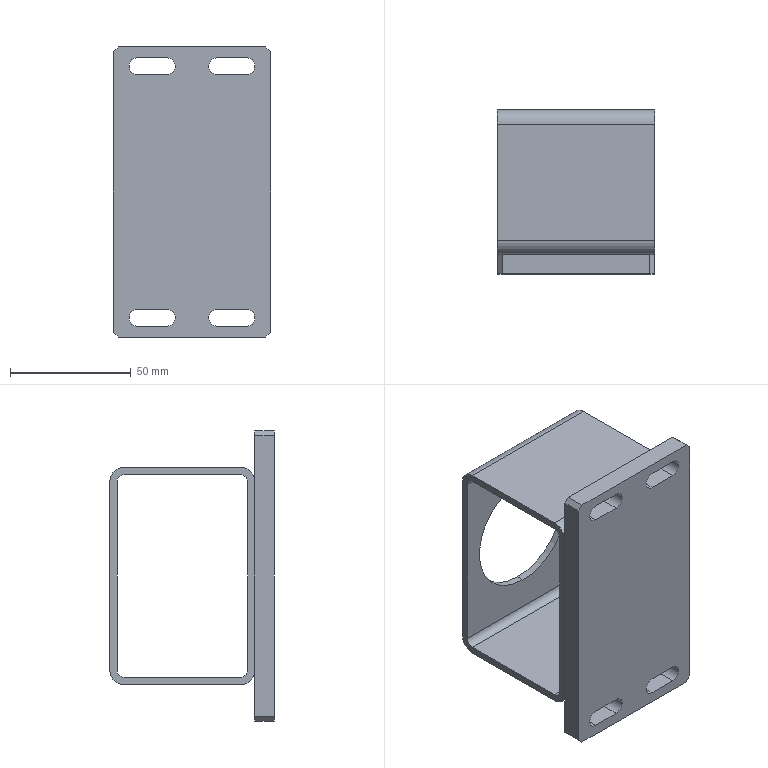Part | SolidWorks | features ICE 5, MirrorPattern 3, Chamfer 1, WeldMemberFeat 1, WeldmentFeature 1 | 2 solids | 46 faces | box 65 x 68 x 120 mm | volume 106942 mm3 | plane 28 | cylinder 18 | commonest cylinder face diameters 7 x8 6 x4 12 x4 51 x2
STEP:
#1=CARTESIAN_POINT('',(0.,27.,-25.5));
#2=VERTEX_POINT('',#1);
#3=CARTESIAN_POINT('',(0.,27.,25.5));
#4=VERTEX_POINT('',#3);
#5=CARTESIAN_POINT('',(0.,27.,0.));
#6=DIRECTION('',(0.,1.,0.));
#7=DIRECTION('',(1.,0.,0.));
#8=AXIS2_PLACEMENT_3D('',#5,#6,#7);
#9=CIRCLE('',#8,25.5);
#10=EDGE_CURVE('',#2,#4,#9,.T.);
#11=ORIENTED_EDGE('',*,*,#10,.F.);
#12=CARTESIAN_POINT('',(0.,30.,-25.5));
#13=VERTEX_POINT('',#12);
#14=CARTESIAN_POINT('',(0.,-30.001,-25.5));
#15=DIRECTION('',(0.,1.,0.));
#16=VECTOR('',#15,1000.);
#17=LINE('',#14,#16);
#18=EDGE_CURVE('',#2,#13,#17,.T.);
#19=ORIENTED_EDGE('',*,*,#18,.T.);
#20=CARTESIAN_POINT('',(0.,30.,25.5));
#21=VERTEX_POINT('',#20);
#22=CARTESIAN_POINT('',(0.,30.,0.));
#23=DIRECTION('',(0.,1.,0.));
#24=DIRECTION('',(0.,0.,1.));
#25=AXIS2_PLACEMENT_3D('',#22,#23,#24);
#26=CIRCLE('',#25,25.5);
#27=EDGE_CURVE('',#13,#21,#26,.T.);
#28=ORIENTED_EDGE('',*,*,#27,.T.);
#29=CARTESIAN_POINT('',(0.,-30.001,25.5));
#30=DIRECTION('',(0.,1.,0.));
#31=VECTOR('',#30,1000.);
#32=LINE('',#29,#31);
#33=EDGE_CURVE('',#4,#21,#32,.T.);
#34=ORIENTED_EDGE('',*,*,#33,.F.);
#35=EDGE_LOOP('',(#11,#19,#28,#34));
#36=FACE_OUTER_BOUND('',#35,.T.);
#37=CARTESIAN_POINT('',(0.,-30.001,0.));
#38=DIRECTION('',(0.,1.,0.));
#39=DIRECTION('',(0.,0.,1.));
#40=AXIS2_PLACEMENT_3D('',#37,#38,#39);
#41=CYLINDRICAL_SURFACE('',#40,25.5);
#42=ADVANCED_FACE('',(#36),#41,.F.);
#43=CARTESIAN_POINT('',(-32.5,30.,39.));
#44=VERTEX_POINT('',#43);
#45=CARTESIAN_POINT('',(-32.5,24.,45.));
#46=VERTEX_POINT('',#45);
#47=CARTESIAN_POINT('',(-32.5,24.,39.));
#48=DIRECTION('',(1.,0.,0.));
#49=DIRECTION('',(0.,1.,0.));
#50=AXIS2_PLACEMENT_3D('',#47,#48,#49);
#51=CIRCLE('',#50,6.);
#52=EDGE_CURVE('',#44,#46,#51,.T.);
#53=ORIENTED_EDGE('',*,*,#52,.T.);
#54=CARTESIAN_POINT('',(32.5,24.,45.));
#55=VERTEX_POINT('',#54);
#56=CARTESIAN_POINT('',(32.5,24.,45.));
#57=DIRECTION('',(-1.,0.,0.));
#58=VECTOR('',#57,1000.);
#59=LINE('',#56,#58);
#60=EDGE_CURVE('',#55,#46,#59,.T.);
#61=ORIENTED_EDGE('',*,*,#60,.F.);
#62=CARTESIAN_POINT('',(32.5,30.,39.));
#63=VERTEX_POINT('',#62);
#64=CARTESIAN_POINT('',(32.5,24.,39.));
#65=DIRECTION('',(1.,0.,0.));
#66=DIRECTION('',(0.,1.,0.));
#67=AXIS2_PLACEMENT_3D('',#64,#65,#66);
#68=CIRCLE('',#67,6.);
#69=EDGE_CURVE('',#63,#55,#68,.T.);
#70=ORIENTED_EDGE('',*,*,#69,.F.);
#71=CARTESIAN_POINT('',(32.5,30.,39.));
#72=DIRECTION('',(-1.,0.,0.));
#73=VECTOR('',#72,1000.);
#74=LINE('',#71,#73);
#75=EDGE_CURVE('',#63,#44,#74,.T.);
#76=ORIENTED_EDGE('',*,*,#75,.T.);
#77=EDGE_LOOP('',(#53,#61,#70,#76));
#78=FACE_OUTER_BOUND('',#77,.T.);
#79=CARTESIAN_POINT('',(32.5,24.,39.));
#80=DIRECTION('',(-1.,0.,0.));
#81=DIRECTION('',(0.,-1.,0.));
#82=AXIS2_PLACEMENT_3D('',#79,#80,#81);
#83=CYLINDRICAL_SURFACE('',#82,6.);
#84=ADVANCED_FACE('',(#78),#83,.T.);
#85=CARTESIAN_POINT('',(-32.5,-24.,45.));
#86=VERTEX_POINT('',#85);
#87=CARTESIAN_POINT('',(-32.5,24.,45.));
#88=DIRECTION('',(0.,-1.,0.));
#89=VECTOR('',#88,1000.);
#90=LINE('',#87,#89);
#91=EDGE_CURVE('',#46,#86,#90,.T.);
#92=ORIENTED_EDGE('',*,*,#91,.T.);
#93=CARTESIAN_POINT('',(32.5,-24.,45.));
#94=VERTEX_POINT('',#93);
#95=CARTESIAN_POINT('',(32.5,-24.,45.));
#96=DIRECTION('',(-1.,0.,0.));
#97=VECTOR('',#96,1000.);
#98=LINE('',#95,#97);
#99=EDGE_CURVE('',#94,#86,#98,.T.);
#100=ORIENTED_EDGE('',*,*,#99,.F.);
#101=CARTESIAN_POINT('',(32.5,24.,45.));
#102=DIRECTION('',(0.,-1.,0.));
#103=VECTOR('',#102,1000.);
#104=LINE('',#101,#103);
#105=EDGE_CURVE('',#55,#94,#104,.T.);
#106=ORIENTED_EDGE('',*,*,#105,.F.);
#107=ORIENTED_EDGE('',*,*,#60,.T.);
#108=EDGE_LOOP('',(#92,#100,#106,#107));
#109=FACE_OUTER_BOUND('',#108,.T.);
#110=CARTESIAN_POINT('',(32.5,24.,45.));
#111=DIRECTION('',(0.,0.,-1.));
#112=DIRECTION('',(-1.,0.,0.));
#113=AXIS2_PLACEMENT_3D('',#110,#111,#112);
#114=PLANE('',#113);
#115=ADVANCED_FACE('',(#109),#114,.F.);
#116=CARTESIAN_POINT('',(-32.5,-30.,39.));
#117=VERTEX_POINT('',#116);
#118=CARTESIAN_POINT('',(-32.5,-24.,39.));
#119=DIRECTION('',(1.,0.,0.));
#120=DIRECTION('',(0.,1.,0.));
#121=AXIS2_PLACEMENT_3D('',#118,#119,#120);
#122=CIRCLE('',#121,6.);
#123=EDGE_CURVE('',#86,#117,#122,.T.);
#124=ORIENTED_EDGE('',*,*,#123,.T.);
#125=CARTESIAN_POINT('',(32.5,-30.,39.));
#126=VERTEX_POINT('',#125);
#127=CARTESIAN_POINT('',(32.5,-30.,39.));
#128=DIRECTION('',(-1.,0.,0.));
#129=VECTOR('',#128,1000.);
#130=LINE('',#127,#129);
#131=EDGE_CURVE('',#126,#117,#130,.T.);
#132=ORIENTED_EDGE('',*,*,#131,.F.);
#133=CARTESIAN_POINT('',(32.5,-24.,39.));
#134=DIRECTION('',(1.,0.,0.));
#135=DIRECTION('',(0.,1.,0.));
#136=AXIS2_PLACEMENT_3D('',#133,#134,#135);
#137=CIRCLE('',#136,6.);
#138=EDGE_CURVE('',#94,#126,#137,.T.);
#139=ORIENTED_EDGE('',*,*,#138,.F.);
#140=ORIENTED_EDGE('',*,*,#99,.T.);
#141=EDGE_LOOP('',(#124,#132,#139,#140));
#142=FACE_OUTER_BOUND('',#141,.T.);
#143=CARTESIAN_POINT('',(32.5,-24.,39.));
#144=DIRECTION('',(-1.,0.,0.));
#145=DIRECTION('',(0.,-1.,0.));
#146=AXIS2_PLACEMENT_3D('',#143,#144,#145);
#147=CYLINDRICAL_SURFACE('',#146,6.);
#148=ADVANCED_FACE('',(#142),#147,.T.);
#149=CARTESIAN_POINT('',(-32.5,-30.,-39.));
#150=VERTEX_POINT('',#149);
#151=CARTESIAN_POINT('',(-32.5,-30.,-39.));
#152=DIRECTION('',(0.,0.,-1.));
#153=VECTOR('',#152,1000.);
#154=LINE('',#151,#153);
#155=EDGE_CURVE('',#117,#150,#154,.T.);
#156=ORIENTED_EDGE('',*,*,#155,.T.);
#157=CARTESIAN_POINT('',(32.5,-30.,-39.));
#158=VERTEX_POINT('',#157);
#159=CARTESIAN_POINT('',(32.5,-30.,-39.));
#160=DIRECTION('',(-1.,0.,0.));
#161=VECTOR('',#160,1000.);
#162=LINE('',#159,#161);
#163=EDGE_CURVE('',#158,#150,#162,.T.);
#164=ORIENTED_EDGE('',*,*,#163,.F.);
#165=CARTESIAN_POINT('',(32.5,-30.,-39.));
#166=DIRECTION('',(0.,0.,-1.));
#167=VECTOR('',#166,1000.);
#168=LINE('',#165,#167);
#169=EDGE_CURVE('',#126,#158,#168,.T.);
#170=ORIENTED_EDGE('',*,*,#169,.F.);
#171=ORIENTED_EDGE('',*,*,#131,.T.);
#172=EDGE_LOOP('',(#156,#164,#170,#171));
#173=FACE_OUTER_BOUND('',#172,.T.);
#174=CARTESIAN_POINT('',(32.5,-30.,-39.));
#175=DIRECTION('',(0.,1.,0.));
#176=DIRECTION('',(-1.,0.,0.));
#177=AXIS2_PLACEMENT_3D('',#174,#175,#176);
#178=PLANE('',#177);
#179=ADVANCED_FACE('',(#173),#178,.F.);
#180=CARTESIAN_POINT('',(-32.5,-24.,-45.));
#181=VERTEX_POINT('',#180);
#182=CARTESIAN_POINT('',(-32.5,-24.,-39.));
#183=DIRECTION('',(1.,0.,0.));
#184=DIRECTION('',(0.,1.,0.));
#185=AXIS2_PLACEMENT_3D('',#182,#183,#184);
#186=CIRCLE('',#185,6.);
#187=EDGE_CURVE('',#150,#181,#186,.T.);
#188=ORIENTED_EDGE('',*,*,#187,.T.);
#189=CARTESIAN_POINT('',(32.5,-24.,-45.));
#190=VERTEX_POINT('',#189);
#191=CARTESIAN_POINT('',(32.5,-24.,-45.));
#192=DIRECTION('',(-1.,0.,0.));
#193=VECTOR('',#192,1000.);
#194=LINE('',#191,#193);
#195=EDGE_CURVE('',#190,#181,#194,.T.);
#196=ORIENTED_EDGE('',*,*,#195,.F.);
#197=CARTESIAN_POINT('',(32.5,-24.,-39.));
#198=DIRECTION('',(1.,0.,0.));
#199=DIRECTION('',(0.,1.,0.));
#200=AXIS2_PLACEMENT_3D('',#197,#198,#199);
#201=CIRCLE('',#200,6.);
#202=EDGE_CURVE('',#158,#190,#201,.T.);
#203=ORIENTED_EDGE('',*,*,#202,.F.);
#204=ORIENTED_EDGE('',*,*,#163,.T.);
#205=EDGE_LOOP('',(#188,#196,#203,#204));
#206=FACE_OUTER_BOUND('',#205,.T.);
#207=CARTESIAN_POINT('',(32.5,-24.,-39.));
#208=DIRECTION('',(-1.,0.,0.));
#209=DIRECTION('',(0.,-1.,0.));
#210=AXIS2_PLACEMENT_3D('',#207,#208,#209);
#211=CYLINDRICAL_SURFACE('',#210,6.);
#212=ADVANCED_FACE('',(#206),#211,.T.);
#213=CARTESIAN_POINT('',(-32.5,24.,-45.));
#214=VERTEX_POINT('',#213);
#215=CARTESIAN_POINT('',(-32.5,-24.,-45.));
#216=DIRECTION('',(0.,1.,0.));
#217=VECTOR('',#216,1000.);
#218=LINE('',#215,#217);
#219=EDGE_CURVE('',#181,#214,#218,.T.);
#220=ORIENTED_EDGE('',*,*,#219,.T.);
#221=CARTESIAN_POINT('',(32.5,24.,-45.));
#222=VERTEX_POINT('',#221);
#223=CARTESIAN_POINT('',(32.5,24.,-45.));
#224=DIRECTION('',(-1.,0.,0.));
#225=VECTOR('',#224,1000.);
#226=LINE('',#223,#225);
#227=EDGE_CURVE('',#222,#214,#226,.T.);
#228=ORIENTED_EDGE('',*,*,#227,.F.);
#229=CARTESIAN_POINT('',(32.5,-24.,-45.));
#230=DIRECTION('',(0.,1.,0.));
#231=VECTOR('',#230,1000.);
#232=LINE('',#229,#231);
#233=EDGE_CURVE('',#190,#222,#232,.T.);
#234=ORIENTED_EDGE('',*,*,#233,.F.);
#235=ORIENTED_EDGE('',*,*,#195,.T.);
#236=EDGE_LOOP('',(#220,#228,#234,#235));
#237=FACE_OUTER_BOUND('',#236,.T.);
#238=CARTESIAN_POINT('',(32.5,-24.,-45.));
#239=DIRECTION('',(0.,0.,1.));
#240=DIRECTION('',(1.,0.,0.));
#241=AXIS2_PLACEMENT_3D('',#238,#239,#240);
#242=PLANE('',#241);
#243=ADVANCED_FACE('',(#237),#242,.F.);
#244=CARTESIAN_POINT('',(-32.5,30.,-39.));
#245=VERTEX_POINT('',#244);
#246=CARTESIAN_POINT('',(-32.5,24.,-39.));
#247=DIRECTION('',(1.,0.,0.));
#248=DIRECTION('',(0.,1.,0.));
#249=AXIS2_PLACEMENT_3D('',#246,#247,#248);
#250=CIRCLE('',#249,6.);
#251=EDGE_CURVE('',#214,#245,#250,.T.);
#252=ORIENTED_EDGE('',*,*,#251,.T.);
#253=CARTESIAN_POINT('',(32.5,30.,-39.));
#254=VERTEX_POINT('',#253);
#255=CARTESIAN_POINT('',(32.5,30.,-39.));
#256=DIRECTION('',(-1.,0.,0.));
#257=VECTOR('',#256,1000.);
#258=LINE('',#255,#257);
#259=EDGE_CURVE('',#254,#245,#258,.T.);
#260=ORIENTED_EDGE('',*,*,#259,.F.);
#261=CARTESIAN_POINT('',(32.5,24.,-39.));
#262=DIRECTION('',(1.,0.,0.));
#263=DIRECTION('',(0.,1.,0.));
#264=AXIS2_PLACEMENT_3D('',#261,#262,#263);
#265=CIRCLE('',#264,6.);
#266=EDGE_CURVE('',#222,#254,#265,.T.);
#267=ORIENTED_EDGE('',*,*,#266,.F.);
#268=ORIENTED_EDGE('',*,*,#227,.T.);
#269=EDGE_LOOP('',(#252,#260,#267,#268));
#270=FACE_OUTER_BOUND('',#269,.T.);
#271=CARTESIAN_POINT('',(32.5,24.,-39.));
#272=DIRECTION('',(-1.,0.,0.));
#273=DIRECTION('',(0.,-1.,0.));
#274=AXIS2_PLACEMENT_3D('',#271,#272,#273);
#275=CYLINDRICAL_SURFACE('',#274,6.);
#276=ADVANCED_FACE('',(#270),#275,.T.);
#277=CARTESIAN_POINT('',(-32.5,-24.,42.));
#278=VERTEX_POINT('',#277);
#279=CARTESIAN_POINT('',(-32.5,-27.,39.));
#280=VERTEX_POINT('',#279);
#281=CARTESIAN_POINT('',(-32.5,-24.,39.));
#282=DIRECTION('',(1.,0.,0.));
#283=DIRECTION('',(0.,1.,0.));
#284=AXIS2_PLACEMENT_3D('',#281,#282,#283);
#285=CIRCLE('',#284,3.);
#286=EDGE_CURVE('',#278,#280,#285,.T.);
#287=ORIENTED_EDGE('',*,*,#286,.F.);
#288=CARTESIAN_POINT('',(32.5,-24.,42.));
#289=VERTEX_POINT('',#288);
#290=CARTESIAN_POINT('',(32.5,-24.,42.));
#291=DIRECTION('',(-1.,0.,0.));
#292=VECTOR('',#291,1000.);
#293=LINE('',#290,#292);
#294=EDGE_CURVE('',#289,#278,#293,.T.);
#295=ORIENTED_EDGE('',*,*,#294,.F.);
#296=CARTESIAN_POINT('',(32.5,-27.,39.));
#297=VERTEX_POINT('',#296);
#298=CARTESIAN_POINT('',(32.5,-24.,39.));
#299=DIRECTION('',(1.,0.,0.));
#300=DIRECTION('',(0.,1.,0.));
#301=AXIS2_PLACEMENT_3D('',#298,#299,#300);
#302=CIRCLE('',#301,3.);
#303=EDGE_CURVE('',#289,#297,#302,.T.);
#304=ORIENTED_EDGE('',*,*,#303,.T.);
#305=CARTESIAN_POINT('',(32.5,-27.,39.));
#306=DIRECTION('',(-1.,0.,0.));
#307=VECTOR('',#306,1000.);
#308=LINE('',#305,#307);
#309=EDGE_CURVE('',#297,#280,#308,.T.);
#310=ORIENTED_EDGE('',*,*,#309,.T.);
#311=EDGE_LOOP('',(#287,#295,#304,#310));
#312=FACE_OUTER_BOUND('',#311,.T.);
#313=CARTESIAN_POINT('',(32.5,-24.,39.));
#314=DIRECTION('',(-1.,0.,0.));
#315=DIRECTION('',(0.,-1.,0.));
#316=AXIS2_PLACEMENT_3D('',#313,#314,#315);
#317=CYLINDRICAL_SURFACE('',#316,3.);
#318=ADVANCED_FACE('',(#312),#317,.F.);
#319=CARTESIAN_POINT('',(-32.5,24.,42.));
#320=VERTEX_POINT('',#319);
#321=CARTESIAN_POINT('',(-32.5,24.,42.));
#322=DIRECTION('',(0.,-1.,0.));
#323=VECTOR('',#322,1000.);
#324=LINE('',#321,#323);
#325=EDGE_CURVE('',#320,#278,#324,.T.);
#326=ORIENTED_EDGE('',*,*,#325,.F.);
#327=CARTESIAN_POINT('',(32.5,24.,42.));
#328=VERTEX_POINT('',#327);
#329=CARTESIAN_POINT('',(32.5,24.,42.));
#330=DIRECTION('',(-1.,0.,0.));
#331=VECTOR('',#330,1000.);
#332=LINE('',#329,#331);
#333=EDGE_CURVE('',#328,#320,#332,.T.);
#334=ORIENTED_EDGE('',*,*,#333,.F.);
#335=CARTESIAN_POINT('',(32.5,24.,42.));
#336=DIRECTION('',(0.,-1.,0.));
#337=VECTOR('',#336,1000.);
#338=LINE('',#335,#337);
#339=EDGE_CURVE('',#328,#289,#338,.T.);
#340=ORIENTED_EDGE('',*,*,#339,.T.);
#341=ORIENTED_EDGE('',*,*,#294,.T.);
#342=EDGE_LOOP('',(#326,#334,#340,#341));
#343=FACE_OUTER_BOUND('',#342,.T.);
#344=CARTESIAN_POINT('',(32.5,24.,42.));
#345=DIRECTION('',(0.,0.,-1.));
#346=DIRECTION('',(-1.,0.,0.));
#347=AXIS2_PLACEMENT_3D('',#344,#345,#346);
#348=PLANE('',#347);
#349=ADVANCED_FACE('',(#343),#348,.T.);
#350=CARTESIAN_POINT('',(-32.5,27.,39.));
#351=VERTEX_POINT('',#350);
#352=CARTESIAN_POINT('',(-32.5,24.,39.));
#353=DIRECTION('',(1.,0.,0.));
#354=DIRECTION('',(0.,1.,0.));
#355=AXIS2_PLACEMENT_3D('',#352,#353,#354);
#356=CIRCLE('',#355,3.);
#357=EDGE_CURVE('',#351,#320,#356,.T.);
#358=ORIENTED_EDGE('',*,*,#357,.F.);
#359=CARTESIAN_POINT('',(32.5,27.,39.));
#360=VERTEX_POINT('',#359);
#361=CARTESIAN_POINT('',(32.5,27.,39.));
#362=DIRECTION('',(-1.,0.,0.));
#363=VECTOR('',#362,1000.);
#364=LINE('',#361,#363);
#365=EDGE_CURVE('',#360,#351,#364,.T.);
#366=ORIENTED_EDGE('',*,*,#365,.F.);
#367=CARTESIAN_POINT('',(32.5,24.,39.));
#368=DIRECTION('',(1.,0.,0.));
#369=DIRECTION('',(0.,1.,0.));
#370=AXIS2_PLACEMENT_3D('',#367,#368,#369);
#371=CIRCLE('',#370,3.);
#372=EDGE_CURVE('',#360,#328,#371,.T.);
#373=ORIENTED_EDGE('',*,*,#372,.T.);
#374=ORIENTED_EDGE('',*,*,#333,.T.);
#375=EDGE_LOOP('',(#358,#366,#373,#374));
#376=FACE_OUTER_BOUND('',#375,.T.);
#377=CARTESIAN_POINT('',(32.5,24.,39.));
#378=DIRECTION('',(-1.,0.,0.));
#379=DIRECTION('',(0.,-1.,0.));
#380=AXIS2_PLACEMENT_3D('',#377,#378,#379);
#381=CYLINDRICAL_SURFACE('',#380,3.);
#382=ADVANCED_FACE('',(#376),#381,.F.);
#383=CARTESIAN_POINT('',(0.,27.,0.));
#384=DIRECTION('',(0.,1.,0.));
#385=DIRECTION('',(1.,0.,0.));
#386=AXIS2_PLACEMENT_3D('',#383,#384,#385);
#387=CIRCLE('',#386,25.5);
#388=EDGE_CURVE('',#4,#2,#387,.T.);
#389=ORIENTED_EDGE('',*,*,#388,.T.);
#390=ORIENTED_EDGE('',*,*,#10,.T.);
#391=EDGE_LOOP('',(#389,#390));
#392=FACE_BOUND('',#391,.T.);
#393=CARTESIAN_POINT('',(-32.5,27.,-39.));
#394=VERTEX_POINT('',#393);
#395=CARTESIAN_POINT('',(-32.5,27.,39.));
#396=DIRECTION('',(0.,0.,1.));
#397=VECTOR('',#396,1000.);
#398=LINE('',#395,#397);
#399=EDGE_CURVE('',#394,#351,#398,.T.);
#400=ORIENTED_EDGE('',*,*,#399,.F.);
#401=CARTESIAN_POINT('',(32.5,27.,-39.));
#402=VERTEX_POINT('',#401);
#403=CARTESIAN_POINT('',(32.5,27.,-39.));
#404=DIRECTION('',(-1.,0.,0.));
#405=VECTOR('',#404,1000.);
#406=LINE('',#403,#405);
#407=EDGE_CURVE('',#402,#394,#406,.T.);
#408=ORIENTED_EDGE('',*,*,#407,.F.);
#409=CARTESIAN_POINT('',(32.5,27.,39.));
#410=DIRECTION('',(0.,0.,1.));
#411=VECTOR('',#410,1000.);
#412=LINE('',#409,#411);
#413=EDGE_CURVE('',#402,#360,#412,.T.);
#414=ORIENTED_EDGE('',*,*,#413,.T.);
#415=ORIENTED_EDGE('',*,*,#365,.T.);
#416=EDGE_LOOP('',(#400,#408,#414,#415));
#417=FACE_OUTER_BOUND('',#416,.T.);
#418=CARTESIAN_POINT('',(32.5,27.,39.));
#419=DIRECTION('',(0.,-1.,0.));
#420=DIRECTION('',(1.,0.,0.));
#421=AXIS2_PLACEMENT_3D('',#418,#419,#420);
#422=PLANE('',#421);
#423=ADVANCED_FACE('',(#392,#417),#422,.T.);
#424=CARTESIAN_POINT('',(-32.5,24.,-42.));
#425=VERTEX_POINT('',#424);
#426=CARTESIAN_POINT('',(-32.5,24.,-39.));
#427=DIRECTION('',(1.,0.,0.));
#428=DIRECTION('',(0.,1.,0.));
#429=AXIS2_PLACEMENT_3D('',#426,#427,#428);
#430=CIRCLE('',#429,3.);
#431=EDGE_CURVE('',#425,#394,#430,.T.);
#432=ORIENTED_EDGE('',*,*,#431,.F.);
#433=CARTESIAN_POINT('',(32.5,24.,-42.));
#434=VERTEX_POINT('',#433);
#435=CARTESIAN_POINT('',(32.5,24.,-42.));
#436=DIRECTION('',(-1.,0.,0.));
#437=VECTOR('',#436,1000.);
#438=LINE('',#435,#437);
#439=EDGE_CURVE('',#434,#425,#438,.T.);
#440=ORIENTED_EDGE('',*,*,#439,.F.);
#441=CARTESIAN_POINT('',(32.5,24.,-39.));
#442=DIRECTION('',(1.,0.,0.));
#443=DIRECTION('',(0.,1.,0.));
#444=AXIS2_PLACEMENT_3D('',#441,#442,#443);
#445=CIRCLE('',#444,3.);
#446=EDGE_CURVE('',#434,#402,#445,.T.);
#447=ORIENTED_EDGE('',*,*,#446,.T.);
#448=ORIENTED_EDGE('',*,*,#407,.T.);
#449=EDGE_LOOP('',(#432,#440,#447,#448));
#450=FACE_OUTER_BOUND('',#449,.T.);
#451=CARTESIAN_POINT('',(32.5,24.,-39.));
#452=DIRECTION('',(-1.,0.,0.));
#453=DIRECTION('',(0.,-1.,0.));
#454=AXIS2_PLACEMENT_3D('',#451,#452,#453);
#455=CYLINDRICAL_SURFACE('',#454,3.);
#456=ADVANCED_FACE('',(#450),#455,.F.);
#457=CARTESIAN_POINT('',(-32.5,-24.,-42.));
#458=VERTEX_POINT('',#457);
#459=CARTESIAN_POINT('',(-32.5,-24.,-42.));
#460=DIRECTION('',(0.,1.,0.));
#461=VECTOR('',#460,1000.);
#462=LINE('',#459,#461);
#463=EDGE_CURVE('',#458,#425,#462,.T.);
#464=ORIENTED_EDGE('',*,*,#463,.F.);
#465=CARTESIAN_POINT('',(32.5,-24.,-42.));
#466=VERTEX_POINT('',#465);
#467=CARTESIAN_POINT('',(32.5,-24.,-42.));
#468=DIRECTION('',(-1.,0.,0.));
#469=VECTOR('',#468,1000.);
#470=LINE('',#467,#469);
#471=EDGE_CURVE('',#466,#458,#470,.T.);
#472=ORIENTED_EDGE('',*,*,#471,.F.);
#473=CARTESIAN_POINT('',(32.5,-24.,-42.));
#474=DIRECTION('',(0.,1.,0.));
#475=VECTOR('',#474,1000.);
#476=LINE('',#473,#475);
#477=EDGE_CURVE('',#466,#434,#476,.T.);
#478=ORIENTED_EDGE('',*,*,#477,.T.);
#479=ORIENTED_EDGE('',*,*,#439,.T.);
#480=EDGE_LOOP('',(#464,#472,#478,#479));
#481=FACE_OUTER_BOUND('',#480,.T.);
#482=CARTESIAN_POINT('',(32.5,-24.,-42.));
#483=DIRECTION('',(0.,0.,1.));
#484=DIRECTION('',(1.,0.,0.));
#485=AXIS2_PLACEMENT_3D('',#482,#483,#484);
#486=PLANE('',#485);
#487=ADVANCED_FACE('',(#481),#486,.T.);
#488=CARTESIAN_POINT('',(-32.5,-27.,-39.));
#489=VERTEX_POINT('',#488);
#490=CARTESIAN_POINT('',(-32.5,-24.,-39.));
#491=DIRECTION('',(1.,0.,0.));
#492=DIRECTION('',(0.,1.,0.));
#493=AXIS2_PLACEMENT_3D('',#490,#491,#492);
#494=CIRCLE('',#493,3.);
#495=EDGE_CURVE('',#489,#458,#494,.T.);
#496=ORIENTED_EDGE('',*,*,#495,.F.);
#497=CARTESIAN_POINT('',(32.5,-27.,-39.));
#498=VERTEX_POINT('',#497);
#499=CARTESIAN_POINT('',(32.5,-27.,-39.));
#500=DIRECTION('',(-1.,0.,0.));
#501=VECTOR('',#500,1000.);
#502=LINE('',#499,#501);
#503=EDGE_CURVE('',#498,#489,#502,.T.);
#504=ORIENTED_EDGE('',*,*,#503,.F.);
#505=CARTESIAN_POINT('',(32.5,-24.,-39.));
#506=DIRECTION('',(1.,0.,0.));
#507=DIRECTION('',(0.,1.,0.));
#508=AXIS2_PLACEMENT_3D('',#505,#506,#507);
#509=CIRCLE('',#508,3.);
#510=EDGE_CURVE('',#498,#466,#509,.T.);
#511=ORIENTED_EDGE('',*,*,#510,.T.);
#512=ORIENTED_EDGE('',*,*,#471,.T.);
#513=EDGE_LOOP('',(#496,#504,#511,#512));
#514=FACE_OUTER_BOUND('',#513,.T.);
#515=CARTESIAN_POINT('',(32.5,-24.,-39.));
#516=DIRECTION('',(-1.,0.,0.));
#517=DIRECTION('',(0.,-1.,0.));
#518=AXIS2_PLACEMENT_3D('',#515,#516,#517);
#519=CYLINDRICAL_SURFACE('',#518,3.);
#520=ADVANCED_FACE('',(#514),#519,.F.);
#521=CARTESIAN_POINT('',(-32.5,-27.,-39.));
#522=DIRECTION('',(0.,0.,-1.));
#523=VECTOR('',#522,1000.);
#524=LINE('',#521,#523);
#525=EDGE_CURVE('',#280,#489,#524,.T.);
#526=ORIENTED_EDGE('',*,*,#525,.F.);
#527=ORIENTED_EDGE('',*,*,#309,.F.);
#528=CARTESIAN_POINT('',(32.5,-27.,-39.));
#529=DIRECTION('',(0.,0.,-1.));
#530=VECTOR('',#529,1000.);
#531=LINE('',#528,#530);
#532=EDGE_CURVE('',#297,#498,#531,.T.);
#533=ORIENTED_EDGE('',*,*,#532,.T.);
#534=ORIENTED_EDGE('',*,*,#503,.T.);
#535=EDGE_LOOP('',(#526,#527,#533,#534));
#536=FACE_OUTER_BOUND('',#535,.T.);
#537=CARTESIAN_POINT('',(32.5,-27.,-39.));
#538=DIRECTION('',(0.,1.,0.));
#539=DIRECTION('',(-1.,0.,0.));
#540=AXIS2_PLACEMENT_3D('',#537,#538,#539);
#541=PLANE('',#540);
#542=ADVANCED_FACE('',(#536),#541,.T.);
#543=CARTESIAN_POINT('',(0.,30.,0.));
#544=DIRECTION('',(0.,1.,0.));
#545=DIRECTION('',(0.,0.,1.));
#546=AXIS2_PLACEMENT_3D('',#543,#544,#545);
#547=CIRCLE('',#546,25.5);
#548=EDGE_CURVE('',#21,#13,#547,.T.);
#549=ORIENTED_EDGE('',*,*,#548,.F.);
#550=ORIENTED_EDGE('',*,*,#27,.F.);
#551=EDGE_LOOP('',(#549,#550));
#552=FACE_BOUND('',#551,.T.);
#553=CARTESIAN_POINT('',(-32.5,30.,39.));
#554=DIRECTION('',(0.,0.,1.));
#555=VECTOR('',#554,1000.);
#556=LINE('',#553,#555);
#557=EDGE_CURVE('',#245,#44,#556,.T.);
#558=ORIENTED_EDGE('',*,*,#557,.T.);
#559=ORIENTED_EDGE('',*,*,#75,.F.);
#560=CARTESIAN_POINT('',(32.5,30.,39.));
#561=DIRECTION('',(0.,0.,1.));
#562=VECTOR('',#561,1000.);
#563=LINE('',#560,#562);
#564=EDGE_CURVE('',#254,#63,#563,.T.);
#565=ORIENTED_EDGE('',*,*,#564,.F.);
#566=ORIENTED_EDGE('',*,*,#259,.T.);
#567=EDGE_LOOP('',(#558,#559,#565,#566));
#568=FACE_OUTER_BOUND('',#567,.T.);
#569=CARTESIAN_POINT('',(32.5,30.,39.));
#570=DIRECTION('',(0.,-1.,0.));
#571=DIRECTION('',(1.,0.,0.));
#572=AXIS2_PLACEMENT_3D('',#569,#570,#571);
#573=PLANE('',#572);
#574=ADVANCED_FACE('',(#552,#568),#573,.F.);
#575=ORIENTED_EDGE('',*,*,#303,.F.);
#576=ORIENTED_EDGE('',*,*,#339,.F.);
#577=ORIENTED_EDGE('',*,*,#372,.F.);
#578=ORIENTED_EDGE('',*,*,#413,.F.);
#579=ORIENTED_EDGE('',*,*,#446,.F.);
#580=ORIENTED_EDGE('',*,*,#477,.F.);
#581=ORIENTED_EDGE('',*,*,#510,.F.);
#582=ORIENTED_EDGE('',*,*,#532,.F.);
#583=EDGE_LOOP('',(#575,#576,#577,#578,#579,#580,#581,#582));
#584=FACE_BOUND('',#583,.T.);
#585=ORIENTED_EDGE('',*,*,#69,.T.);
#586=ORIENTED_EDGE('',*,*,#105,.T.);
#587=ORIENTED_EDGE('',*,*,#138,.T.);
#588=ORIENTED_EDGE('',*,*,#169,.T.);
#589=ORIENTED_EDGE('',*,*,#202,.T.);
#590=ORIENTED_EDGE('',*,*,#233,.T.);
#591=ORIENTED_EDGE('',*,*,#266,.T.);
#592=ORIENTED_EDGE('',*,*,#564,.T.);
#593=EDGE_LOOP('',(#585,#586,#587,#588,#589,#590,#591,#592));
#594=FACE_OUTER_BOUND('',#593,.T.);
#595=CARTESIAN_POINT('',(32.5,24.,39.));
#596=DIRECTION('',(1.,0.,0.));
#597=DIRECTION('',(0.,1.,0.));
#598=AXIS2_PLACEMENT_3D('',#595,#596,#597);
#599=PLANE('',#598);
#600=ADVANCED_FACE('',(#584,#594),#599,.T.);
#601=ORIENTED_EDGE('',*,*,#286,.T.);
#602=ORIENTED_EDGE('',*,*,#525,.T.);
#603=ORIENTED_EDGE('',*,*,#495,.T.);
#604=ORIENTED_EDGE('',*,*,#463,.T.);
#605=ORIENTED_EDGE('',*,*,#431,.T.);
#606=ORIENTED_EDGE('',*,*,#399,.T.);
#607=ORIENTED_EDGE('',*,*,#357,.T.);
#608=ORIENTED_EDGE('',*,*,#325,.T.);
#609=EDGE_LOOP('',(#601,#602,#603,#604,#605,#606,#607,#608));
#610=FACE_BOUND('',#609,.T.);
#611=ORIENTED_EDGE('',*,*,#52,.F.);
#612=ORIENTED_EDGE('',*,*,#557,.F.);
#613=ORIENTED_EDGE('',*,*,#251,.F.);
#614=ORIENTED_EDGE('',*,*,#219,.F.);
#615=ORIENTED_EDGE('',*,*,#187,.F.);
#616=ORIENTED_EDGE('',*,*,#155,.F.);
#617=ORIENTED_EDGE('',*,*,#123,.F.);
#618=ORIENTED_EDGE('',*,*,#91,.F.);
#619=EDGE_LOOP('',(#611,#612,#613,#614,#615,#616,#617,#618));
#620=FACE_OUTER_BOUND('',#619,.T.);
#621=CARTESIAN_POINT('',(-32.5,24.,39.));
#622=DIRECTION('',(1.,0.,0.));
#623=DIRECTION('',(0.,1.,0.));
#624=AXIS2_PLACEMENT_3D('',#621,#622,#623);
#625=PLANE('',#624);
#626=ADVANCED_FACE('',(#610,#620),#625,.F.);
#627=ORIENTED_EDGE('',*,*,#18,.F.);
#628=ORIENTED_EDGE('',*,*,#388,.F.);
#629=ORIENTED_EDGE('',*,*,#33,.T.);
#630=ORIENTED_EDGE('',*,*,#548,.T.);
#631=EDGE_LOOP('',(#627,#628,#629,#630));
#632=FACE_OUTER_BOUND('',#631,.T.);
#633=CARTESIAN_POINT('',(0.,-30.001,0.));
#634=DIRECTION('',(0.,1.,0.));
#635=DIRECTION('',(0.,0.,1.));
#636=AXIS2_PLACEMENT_3D('',#633,#634,#635);
#637=CYLINDRICAL_SURFACE('',#636,25.5);
#638=ADVANCED_FACE('',(#632),#637,.F.);
#639=CLOSED_SHELL('',(#42,#84,#115,#148,#179,#212,#243,#276,#318,#349,#382,#423,#456,#487,#520,#542,#574,#600,#626,#638));
#640=MANIFOLD_SOLID_BREP('',#639);
#641=CARTESIAN_POINT('',(32.5,-38.,-58.));
#642=VERTEX_POINT('',#641);
#643=CARTESIAN_POINT('',(32.5,-38.,58.));
#644=VERTEX_POINT('',#643);
#645=CARTESIAN_POINT('',(32.5,-38.,-60.));
#646=DIRECTION('',(0.,0.,1.));
#647=VECTOR('',#646,1000.);
#648=LINE('',#645,#647);
#649=EDGE_CURVE('',#642,#644,#648,.T.);
#650=ORIENTED_EDGE('',*,*,#649,.F.);
#651=CARTESIAN_POINT('',(32.5,-30.,-58.));
#652=VERTEX_POINT('',#651);
#653=CARTESIAN_POINT('',(32.5,-38.,-58.));
#654=DIRECTION('',(0.,1.,0.));
#655=VECTOR('',#654,1000.);
#656=LINE('',#653,#655);
#657=EDGE_CURVE('',#642,#652,#656,.T.);
#658=ORIENTED_EDGE('',*,*,#657,.T.);
#659=CARTESIAN_POINT('',(32.5,-30.,58.));
#660=VERTEX_POINT('',#659);
#661=CARTESIAN_POINT('',(32.5,-30.,-60.));
#662=DIRECTION('',(0.,0.,1.));
#663=VECTOR('',#662,1000.);
#664=LINE('',#661,#663);
#665=EDGE_CURVE('',#652,#660,#664,.T.);
#666=ORIENTED_EDGE('',*,*,#665,.T.);
#667=CARTESIAN_POINT('',(32.5,-38.,58.));
#668=DIRECTION('',(0.,-1.,0.));
#669=VECTOR('',#668,1000.);
#670=LINE('',#667,#669);
#671=EDGE_CURVE('',#660,#644,#670,.T.);
#672=ORIENTED_EDGE('',*,*,#671,.T.);
#673=EDGE_LOOP('',(#650,#658,#666,#672));
#674=FACE_OUTER_BOUND('',#673,.T.);
#675=CARTESIAN_POINT('',(32.5,-38.,-60.));
#676=DIRECTION('',(-1.,0.,0.));
#677=DIRECTION('',(0.,0.,1.));
#678=AXIS2_PLACEMENT_3D('',#675,#676,#677);
#679=PLANE('',#678);
#680=ADVANCED_FACE('',(#674),#679,.F.);
#681=CARTESIAN_POINT('',(30.5,-38.,60.));
#682=VERTEX_POINT('',#681);
#683=CARTESIAN_POINT('',(-30.5,-38.,60.));
#684=VERTEX_POINT('',#683);
#685=CARTESIAN_POINT('',(-32.5,-38.,60.));
#686=DIRECTION('',(-1.,0.,0.));
#687=VECTOR('',#686,1000.);
#688=LINE('',#685,#687);
#689=EDGE_CURVE('',#682,#684,#688,.T.);
#690=ORIENTED_EDGE('',*,*,#689,.F.);
#691=CARTESIAN_POINT('',(30.5,-30.,60.));
#692=VERTEX_POINT('',#691);
#693=CARTESIAN_POINT('',(30.5,-38.,60.));
#694=DIRECTION('',(0.,1.,0.));
#695=VECTOR('',#694,1000.);
#696=LINE('',#693,#695);
#697=EDGE_CURVE('',#682,#692,#696,.T.);
#698=ORIENTED_EDGE('',*,*,#697,.T.);
#699=CARTESIAN_POINT('',(-30.5,-30.,60.));
#700=VERTEX_POINT('',#699);
#701=CARTESIAN_POINT('',(-32.5,-30.,60.));
#702=DIRECTION('',(-1.,0.,0.));
#703=VECTOR('',#702,1000.);
#704=LINE('',#701,#703);
#705=EDGE_CURVE('',#692,#700,#704,.T.);
#706=ORIENTED_EDGE('',*,*,#705,.T.);
#707=CARTESIAN_POINT('',(-30.5,-38.,60.));
#708=DIRECTION('',(0.,-1.,0.));
#709=VECTOR('',#708,1000.);
#710=LINE('',#707,#709);
#711=EDGE_CURVE('',#700,#684,#710,.T.);
#712=ORIENTED_EDGE('',*,*,#711,.T.);
#713=EDGE_LOOP('',(#690,#698,#706,#712));
#714=FACE_OUTER_BOUND('',#713,.T.);
#715=CARTESIAN_POINT('',(-32.5,-38.,60.));
#716=DIRECTION('',(0.,0.,-1.));
#717=DIRECTION('',(-1.,0.,0.));
#718=AXIS2_PLACEMENT_3D('',#715,#716,#717);
#719=PLANE('',#718);
#720=ADVANCED_FACE('',(#714),#719,.F.);
#721=CARTESIAN_POINT('',(-32.5,-30.,58.));
#722=VERTEX_POINT('',#721);
#723=CARTESIAN_POINT('',(-32.5,-30.,-58.));
#724=VERTEX_POINT('',#723);
#725=CARTESIAN_POINT('',(-32.5,-30.,-60.));
#726=DIRECTION('',(0.,0.,-1.));
#727=VECTOR('',#726,1000.);
#728=LINE('',#725,#727);
#729=EDGE_CURVE('',#722,#724,#728,.T.);
#730=ORIENTED_EDGE('',*,*,#729,.T.);
#731=CARTESIAN_POINT('',(-32.5,-38.,-58.));
#732=VERTEX_POINT('',#731);
#733=CARTESIAN_POINT('',(-32.5,-38.,-58.));
#734=DIRECTION('',(0.,-1.,0.));
#735=VECTOR('',#734,1000.);
#736=LINE('',#733,#735);
#737=EDGE_CURVE('',#724,#732,#736,.T.);
#738=ORIENTED_EDGE('',*,*,#737,.T.);
#739=CARTESIAN_POINT('',(-32.5,-38.,58.));
#740=VERTEX_POINT('',#739);
#741=CARTESIAN_POINT('',(-32.5,-38.,-60.));
#742=DIRECTION('',(0.,0.,-1.));
#743=VECTOR('',#742,1000.);
#744=LINE('',#741,#743);
#745=EDGE_CURVE('',#740,#732,#744,.T.);
#746=ORIENTED_EDGE('',*,*,#745,.F.);
#747=CARTESIAN_POINT('',(-32.5,-38.,58.));
#748=DIRECTION('',(0.,1.,0.));
#749=VECTOR('',#748,1000.);
#750=LINE('',#747,#749);
#751=EDGE_CURVE('',#740,#722,#750,.T.);
#752=ORIENTED_EDGE('',*,*,#751,.T.);
#753=EDGE_LOOP('',(#730,#738,#746,#752));
#754=FACE_OUTER_BOUND('',#753,.T.);
#755=CARTESIAN_POINT('',(-32.5,-38.,-60.));
#756=DIRECTION('',(1.,0.,0.));
#757=DIRECTION('',(0.,0.,-1.));
#758=AXIS2_PLACEMENT_3D('',#755,#756,#757);
#759=PLANE('',#758);
#760=ADVANCED_FACE('',(#754),#759,.F.);
#761=CARTESIAN_POINT('',(-30.5,-30.,-60.));
#762=VERTEX_POINT('',#761);
#763=CARTESIAN_POINT('',(30.5,-30.,-60.));
#764=VERTEX_POINT('',#763);
#765=CARTESIAN_POINT('',(-32.5,-30.,-60.));
#766=DIRECTION('',(1.,0.,0.));
#767=VECTOR('',#766,1000.);
#768=LINE('',#765,#767);
#769=EDGE_CURVE('',#762,#764,#768,.T.);
#770=ORIENTED_EDGE('',*,*,#769,.T.);
#771=CARTESIAN_POINT('',(30.5,-38.,-60.));
#772=VERTEX_POINT('',#771);
#773=CARTESIAN_POINT('',(30.5,-38.,-60.));
#774=DIRECTION('',(0.,-1.,0.));
#775=VECTOR('',#774,1000.);
#776=LINE('',#773,#775);
#777=EDGE_CURVE('',#764,#772,#776,.T.);
#778=ORIENTED_EDGE('',*,*,#777,.T.);
#779=CARTESIAN_POINT('',(-30.5,-38.,-60.));
#780=VERTEX_POINT('',#779);
#781=CARTESIAN_POINT('',(-32.5,-38.,-60.));
#782=DIRECTION('',(1.,0.,0.));
#783=VECTOR('',#782,1000.);
#784=LINE('',#781,#783);
#785=EDGE_CURVE('',#780,#772,#784,.T.);
#786=ORIENTED_EDGE('',*,*,#785,.F.);
#787=CARTESIAN_POINT('',(-30.5,-38.,-60.));
#788=DIRECTION('',(0.,1.,0.));
#789=VECTOR('',#788,1000.);
#790=LINE('',#787,#789);
#791=EDGE_CURVE('',#780,#762,#790,.T.);
#792=ORIENTED_EDGE('',*,*,#791,.T.);
#793=EDGE_LOOP('',(#770,#778,#786,#792));
#794=FACE_OUTER_BOUND('',#793,.T.);
#795=CARTESIAN_POINT('',(-32.5,-38.,-60.));
#796=DIRECTION('',(0.,0.,1.));
#797=DIRECTION('',(1.,0.,0.));
#798=AXIS2_PLACEMENT_3D('',#795,#796,#797);
#799=PLANE('',#798);
#800=ADVANCED_FACE('',(#794),#799,.F.);
#801=CARTESIAN_POINT('',(-22.5,-38.,-55.5));
#802=VERTEX_POINT('',#801);
#803=CARTESIAN_POINT('',(-22.5,-38.,-48.5));
#804=VERTEX_POINT('',#803);
#805=CARTESIAN_POINT('',(-22.5,-38.,-52.));
#806=DIRECTION('',(0.,1.,0.));
#807=DIRECTION('',(0.,0.,1.));
#808=AXIS2_PLACEMENT_3D('',#805,#806,#807);
#809=CIRCLE('',#808,3.5);
#810=EDGE_CURVE('',#802,#804,#809,.T.);
#811=ORIENTED_EDGE('',*,*,#810,.T.);
#812=CARTESIAN_POINT('',(-10.5,-38.,-48.5));
#813=VERTEX_POINT('',#812);
#814=CARTESIAN_POINT('',(-22.5,-38.,-48.5));
#815=DIRECTION('',(1.,0.,0.));
#816=VECTOR('',#815,1000.);
#817=LINE('',#814,#816);
#818=EDGE_CURVE('',#804,#813,#817,.T.);
#819=ORIENTED_EDGE('',*,*,#818,.T.);
#820=CARTESIAN_POINT('',(-10.5,-38.,-55.5));
#821=VERTEX_POINT('',#820);
#822=CARTESIAN_POINT('',(-10.5,-38.,-52.));
#823=DIRECTION('',(0.,1.,0.));
#824=DIRECTION('',(0.,0.,1.));
#825=AXIS2_PLACEMENT_3D('',#822,#823,#824);
#826=CIRCLE('',#825,3.5);
#827=EDGE_CURVE('',#813,#821,#826,.T.);
#828=ORIENTED_EDGE('',*,*,#827,.T.);
#829=CARTESIAN_POINT('',(-22.5,-38.,-55.5));
#830=DIRECTION('',(-1.,0.,0.));
#831=VECTOR('',#830,1000.);
#832=LINE('',#829,#831);
#833=EDGE_CURVE('',#821,#802,#832,.T.);
#834=ORIENTED_EDGE('',*,*,#833,.T.);
#835=EDGE_LOOP('',(#811,#819,#828,#834));
#836=FACE_BOUND('',#835,.T.);
#837=CARTESIAN_POINT('',(10.5,-38.,-48.5));
#838=VERTEX_POINT('',#837);
#839=CARTESIAN_POINT('',(10.5,-38.,-55.5));
#840=VERTEX_POINT('',#839);
#841=CARTESIAN_POINT('',(10.5,-38.,-52.));
#842=DIRECTION('',(0.,-1.,0.));
#843=DIRECTION('',(0.,0.,1.));
#844=AXIS2_PLACEMENT_3D('',#841,#842,#843);
#845=CIRCLE('',#844,3.5);
#846=EDGE_CURVE('',#838,#840,#845,.T.);
#847=ORIENTED_EDGE('',*,*,#846,.F.);
#848=CARTESIAN_POINT('',(22.5,-38.,-48.5));
#849=VERTEX_POINT('',#848);
#850=CARTESIAN_POINT('',(22.5,-38.,-48.5));
#851=DIRECTION('',(-1.,0.,0.));
#852=VECTOR('',#851,1000.);
#853=LINE('',#850,#852);
#854=EDGE_CURVE('',#849,#838,#853,.T.);
#855=ORIENTED_EDGE('',*,*,#854,.F.);
#856=CARTESIAN_POINT('',(22.5,-38.,-55.5));
#857=VERTEX_POINT('',#856);
#858=CARTESIAN_POINT('',(22.5,-38.,-52.));
#859=DIRECTION('',(0.,-1.,0.));
#860=DIRECTION('',(0.,0.,1.));
#861=AXIS2_PLACEMENT_3D('',#858,#859,#860);
#862=CIRCLE('',#861,3.5);
#863=EDGE_CURVE('',#857,#849,#862,.T.);
#864=ORIENTED_EDGE('',*,*,#863,.F.);
#865=CARTESIAN_POINT('',(22.5,-38.,-55.5));
#866=DIRECTION('',(1.,0.,0.));
#867=VECTOR('',#866,1000.);
#868=LINE('',#865,#867);
#869=EDGE_CURVE('',#840,#857,#868,.T.);
#870=ORIENTED_EDGE('',*,*,#869,.F.);
#871=EDGE_LOOP('',(#847,#855,#864,#870));
#872=FACE_BOUND('',#871,.T.);
#873=CARTESIAN_POINT('',(22.5,-38.,55.5));
#874=VERTEX_POINT('',#873);
#875=CARTESIAN_POINT('',(22.5,-38.,48.5));
#876=VERTEX_POINT('',#875);
#877=CARTESIAN_POINT('',(22.5,-38.,52.));
#878=DIRECTION('',(0.,1.,0.));
#879=DIRECTION('',(0.,0.,-1.));
#880=AXIS2_PLACEMENT_3D('',#877,#878,#879);
#881=CIRCLE('',#880,3.5);
#882=EDGE_CURVE('',#874,#876,#881,.T.);
#883=ORIENTED_EDGE('',*,*,#882,.T.);
#884=CARTESIAN_POINT('',(10.5,-38.,48.5));
#885=VERTEX_POINT('',#884);
#886=CARTESIAN_POINT('',(22.5,-38.,48.5));
#887=DIRECTION('',(-1.,0.,0.));
#888=VECTOR('',#887,1000.);
#889=LINE('',#886,#888);
#890=EDGE_CURVE('',#876,#885,#889,.T.);
#891=ORIENTED_EDGE('',*,*,#890,.T.);
#892=CARTESIAN_POINT('',(10.5,-38.,55.5));
#893=VERTEX_POINT('',#892);
#894=CARTESIAN_POINT('',(10.5,-38.,52.));
#895=DIRECTION('',(0.,1.,0.));
#896=DIRECTION('',(0.,0.,-1.));
#897=AXIS2_PLACEMENT_3D('',#894,#895,#896);
#898=CIRCLE('',#897,3.5);
#899=EDGE_CURVE('',#885,#893,#898,.T.);
#900=ORIENTED_EDGE('',*,*,#899,.T.);
#901=CARTESIAN_POINT('',(22.5,-38.,55.5));
#902=DIRECTION('',(1.,0.,0.));
#903=VECTOR('',#902,1000.);
#904=LINE('',#901,#903);
#905=EDGE_CURVE('',#893,#874,#904,.T.);
#906=ORIENTED_EDGE('',*,*,#905,.T.);
#907=EDGE_LOOP('',(#883,#891,#900,#906));
#908=FACE_BOUND('',#907,.T.);
#909=CARTESIAN_POINT('',(-10.5,-38.,48.5));
#910=VERTEX_POINT('',#909);
#911=CARTESIAN_POINT('',(-10.5,-38.,55.5));
#912=VERTEX_POINT('',#911);
#913=CARTESIAN_POINT('',(-10.5,-38.,52.));
#914=DIRECTION('',(0.,-1.,0.));
#915=DIRECTION('',(0.,0.,-1.));
#916=AXIS2_PLACEMENT_3D('',#913,#914,#915);
#917=CIRCLE('',#916,3.5);
#918=EDGE_CURVE('',#910,#912,#917,.T.);
#919=ORIENTED_EDGE('',*,*,#918,.F.);
#920=CARTESIAN_POINT('',(-22.5,-38.,48.5));
#921=VERTEX_POINT('',#920);
#922=CARTESIAN_POINT('',(-22.5,-38.,48.5));
#923=DIRECTION('',(1.,0.,0.));
#924=VECTOR('',#923,1000.);
#925=LINE('',#922,#924);
#926=EDGE_CURVE('',#921,#910,#925,.T.);
#927=ORIENTED_EDGE('',*,*,#926,.F.);
#928=CARTESIAN_POINT('',(-22.5,-38.,55.5));
#929=VERTEX_POINT('',#928);
#930=CARTESIAN_POINT('',(-22.5,-38.,52.));
#931=DIRECTION('',(0.,-1.,0.));
#932=DIRECTION('',(0.,0.,-1.));
#933=AXIS2_PLACEMENT_3D('',#930,#931,#932);
#934=CIRCLE('',#933,3.5);
#935=EDGE_CURVE('',#929,#921,#934,.T.);
#936=ORIENTED_EDGE('',*,*,#935,.F.);
#937=CARTESIAN_POINT('',(-22.5,-38.,55.5));
#938=DIRECTION('',(-1.,0.,0.));
#939=VECTOR('',#938,1000.);
#940=LINE('',#937,#939);
#941=EDGE_CURVE('',#912,#929,#940,.T.);
#942=ORIENTED_EDGE('',*,*,#941,.F.);
#943=EDGE_LOOP('',(#919,#927,#936,#942));
#944=FACE_BOUND('',#943,.T.);
#945=ORIENTED_EDGE('',*,*,#785,.T.);
#946=CARTESIAN_POINT('',(32.5,-38.,-58.));
#947=DIRECTION('',(0.7071,0.,0.7071));
#948=VECTOR('',#947,1000.);
#949=LINE('',#946,#948);
#950=EDGE_CURVE('',#772,#642,#949,.T.);
#951=ORIENTED_EDGE('',*,*,#950,.T.);
#952=ORIENTED_EDGE('',*,*,#649,.T.);
#953=CARTESIAN_POINT('',(30.5,-38.,60.));
#954=DIRECTION('',(-0.7071,0.,0.7071));
#955=VECTOR('',#954,1000.);
#956=LINE('',#953,#955);
#957=EDGE_CURVE('',#644,#682,#956,.T.);
#958=ORIENTED_EDGE('',*,*,#957,.T.);
#959=ORIENTED_EDGE('',*,*,#689,.T.);
#960=CARTESIAN_POINT('',(-32.5,-38.,58.));
#961=DIRECTION('',(-0.7071,0.,-0.7071));
#962=VECTOR('',#961,1000.);
#963=LINE('',#960,#962);
#964=EDGE_CURVE('',#684,#740,#963,.T.);
#965=ORIENTED_EDGE('',*,*,#964,.T.);
#966=ORIENTED_EDGE('',*,*,#745,.T.);
#967=CARTESIAN_POINT('',(-30.5,-38.,-60.));
#968=DIRECTION('',(0.7071,0.,-0.7071));
#969=VECTOR('',#968,1000.);
#970=LINE('',#967,#969);
#971=EDGE_CURVE('',#732,#780,#970,.T.);
#972=ORIENTED_EDGE('',*,*,#971,.T.);
#973=EDGE_LOOP('',(#945,#951,#952,#958,#959,#965,#966,#972));
#974=FACE_OUTER_BOUND('',#973,.T.);
#975=CARTESIAN_POINT('',(0.,-38.,0.));
#976=DIRECTION('',(0.,1.,0.));
#977=DIRECTION('',(0.,0.,1.));
#978=AXIS2_PLACEMENT_3D('',#975,#976,#977);
#979=PLANE('',#978);
#980=ADVANCED_FACE('',(#836,#872,#908,#944,#974),#979,.F.);
#981=CARTESIAN_POINT('',(-10.5,-30.,-48.5));
#982=VERTEX_POINT('',#981);
#983=CARTESIAN_POINT('',(-22.5,-30.,-48.5));
#984=VERTEX_POINT('',#983);
#985=CARTESIAN_POINT('',(0.,-30.,-48.5));
#986=DIRECTION('',(-1.,0.,0.));
#987=VECTOR('',#986,1000.);
#988=LINE('',#985,#987);
#989=EDGE_CURVE('',#982,#984,#988,.T.);
#990=ORIENTED_EDGE('',*,*,#989,.T.);
#991=CARTESIAN_POINT('',(-22.5,-30.,-55.5));
#992=VERTEX_POINT('',#991);
#993=CARTESIAN_POINT('',(-22.5,-30.,-52.));
#994=DIRECTION('',(0.,-1.,0.));
#995=DIRECTION('',(0.,0.,-1.));
#996=AXIS2_PLACEMENT_3D('',#993,#994,#995);
#997=CIRCLE('',#996,3.5);
#998=EDGE_CURVE('',#984,#992,#997,.T.);
#999=ORIENTED_EDGE('',*,*,#998,.T.);
#1000=CARTESIAN_POINT('',(-10.5,-30.,-55.5));
#1001=VERTEX_POINT('',#1000);
#1002=CARTESIAN_POINT('',(0.,-30.,-55.5));
#1003=DIRECTION('',(1.,0.,0.));
#1004=VECTOR('',#1003,1000.);
#1005=LINE('',#1002,#1004);
#1006=EDGE_CURVE('',#992,#1001,#1005,.T.);
#1007=ORIENTED_EDGE('',*,*,#1006,.T.);
#1008=CARTESIAN_POINT('',(-10.5,-30.,-52.));
#1009=DIRECTION('',(0.,-1.,0.));
#1010=DIRECTION('',(0.,0.,-1.));
#1011=AXIS2_PLACEMENT_3D('',#1008,#1009,#1010);
#1012=CIRCLE('',#1011,3.5);
#1013=EDGE_CURVE('',#1001,#982,#1012,.T.);
#1014=ORIENTED_EDGE('',*,*,#1013,.T.);
#1015=EDGE_LOOP('',(#990,#999,#1007,#1014));
#1016=FACE_BOUND('',#1015,.T.);
#1017=CARTESIAN_POINT('',(10.5,-30.,-48.5));
#1018=VERTEX_POINT('',#1017);
#1019=CARTESIAN_POINT('',(22.5,-30.,-48.5));
#1020=VERTEX_POINT('',#1019);
#1021=CARTESIAN_POINT('',(0.,-30.,-48.5));
#1022=DIRECTION('',(1.,0.,0.));
#1023=VECTOR('',#1022,1000.);
#1024=LINE('',#1021,#1023);
#1025=EDGE_CURVE('',#1018,#1020,#1024,.T.);
#1026=ORIENTED_EDGE('',*,*,#1025,.F.);
#1027=CARTESIAN_POINT('',(10.5,-30.,-55.5));
#1028=VERTEX_POINT('',#1027);
#1029=CARTESIAN_POINT('',(10.5,-30.,-52.));
#1030=DIRECTION('',(0.,1.,0.));
#1031=DIRECTION('',(0.,0.,-1.));
#1032=AXIS2_PLACEMENT_3D('',#1029,#1030,#1031);
#1033=CIRCLE('',#1032,3.5);
#1034=EDGE_CURVE('',#1028,#1018,#1033,.T.);
#1035=ORIENTED_EDGE('',*,*,#1034,.F.);
#1036=CARTESIAN_POINT('',(22.5,-30.,-55.5));
#1037=VERTEX_POINT('',#1036);
#1038=CARTESIAN_POINT('',(0.,-30.,-55.5));
#1039=DIRECTION('',(-1.,0.,0.));
#1040=VECTOR('',#1039,1000.);
#1041=LINE('',#1038,#1040);
#1042=EDGE_CURVE('',#1037,#1028,#1041,.T.);
#1043=ORIENTED_EDGE('',*,*,#1042,.F.);
#1044=CARTESIAN_POINT('',(22.5,-30.,-52.));
#1045=DIRECTION('',(0.,1.,0.));
#1046=DIRECTION('',(0.,0.,-1.));
#1047=AXIS2_PLACEMENT_3D('',#1044,#1045,#1046);
#1048=CIRCLE('',#1047,3.5);
#1049=EDGE_CURVE('',#1020,#1037,#1048,.T.);
#1050=ORIENTED_EDGE('',*,*,#1049,.F.);
#1051=EDGE_LOOP('',(#1026,#1035,#1043,#1050));
#1052=FACE_BOUND('',#1051,.T.);
#1053=CARTESIAN_POINT('',(10.5,-30.,48.5));
#1054=VERTEX_POINT('',#1053);
#1055=CARTESIAN_POINT('',(22.5,-30.,48.5));
#1056=VERTEX_POINT('',#1055);
#1057=CARTESIAN_POINT('',(0.,-30.,48.5));
#1058=DIRECTION('',(1.,0.,0.));
#1059=VECTOR('',#1058,1000.);
#1060=LINE('',#1057,#1059);
#1061=EDGE_CURVE('',#1054,#1056,#1060,.T.);
#1062=ORIENTED_EDGE('',*,*,#1061,.T.);
#1063=CARTESIAN_POINT('',(22.5,-30.,55.5));
#1064=VERTEX_POINT('',#1063);
#1065=CARTESIAN_POINT('',(22.5,-30.,52.));
#1066=DIRECTION('',(0.,-1.,0.));
#1067=DIRECTION('',(0.,0.,1.));
#1068=AXIS2_PLACEMENT_3D('',#1065,#1066,#1067);
#1069=CIRCLE('',#1068,3.5);
#1070=EDGE_CURVE('',#1056,#1064,#1069,.T.);
#1071=ORIENTED_EDGE('',*,*,#1070,.T.);
#1072=CARTESIAN_POINT('',(10.5,-30.,55.5));
#1073=VERTEX_POINT('',#1072);
#1074=CARTESIAN_POINT('',(0.,-30.,55.5));
#1075=DIRECTION('',(-1.,0.,0.));
#1076=VECTOR('',#1075,1000.);
#1077=LINE('',#1074,#1076);
#1078=EDGE_CURVE('',#1064,#1073,#1077,.T.);
#1079=ORIENTED_EDGE('',*,*,#1078,.T.);
#1080=CARTESIAN_POINT('',(10.5,-30.,52.));
#1081=DIRECTION('',(0.,-1.,0.));
#1082=DIRECTION('',(0.,0.,1.));
#1083=AXIS2_PLACEMENT_3D('',#1080,#1081,#1082);
#1084=CIRCLE('',#1083,3.5);
#1085=EDGE_CURVE('',#1073,#1054,#1084,.T.);
#1086=ORIENTED_EDGE('',*,*,#1085,.T.);
#1087=EDGE_LOOP('',(#1062,#1071,#1079,#1086));
#1088=FACE_BOUND('',#1087,.T.);
#1089=CARTESIAN_POINT('',(-10.5,-30.,48.5));
#1090=VERTEX_POINT('',#1089);
#1091=CARTESIAN_POINT('',(-22.5,-30.,48.5));
#1092=VERTEX_POINT('',#1091);
#1093=CARTESIAN_POINT('',(0.,-30.,48.5));
#1094=DIRECTION('',(-1.,0.,0.));
#1095=VECTOR('',#1094,1000.);
#1096=LINE('',#1093,#1095);
#1097=EDGE_CURVE('',#1090,#1092,#1096,.T.);
#1098=ORIENTED_EDGE('',*,*,#1097,.F.);
#1099=CARTESIAN_POINT('',(-10.5,-30.,55.5));
#1100=VERTEX_POINT('',#1099);
#1101=CARTESIAN_POINT('',(-10.5,-30.,52.));
#1102=DIRECTION('',(0.,1.,0.));
#1103=DIRECTION('',(0.,0.,1.));
#1104=AXIS2_PLACEMENT_3D('',#1101,#1102,#1103);
#1105=CIRCLE('',#1104,3.5);
#1106=EDGE_CURVE('',#1100,#1090,#1105,.T.);
#1107=ORIENTED_EDGE('',*,*,#1106,.F.);
#1108=CARTESIAN_POINT('',(-22.5,-30.,55.5));
#1109=VERTEX_POINT('',#1108);
#1110=CARTESIAN_POINT('',(0.,-30.,55.5));
#1111=DIRECTION('',(1.,0.,0.));
#1112=VECTOR('',#1111,1000.);
#1113=LINE('',#1110,#1112);
#1114=EDGE_CURVE('',#1109,#1100,#1113,.T.);
#1115=ORIENTED_EDGE('',*,*,#1114,.F.);
#1116=CARTESIAN_POINT('',(-22.5,-30.,52.));
#1117=DIRECTION('',(0.,1.,0.));
#1118=DIRECTION('',(0.,0.,1.));
#1119=AXIS2_PLACEMENT_3D('',#1116,#1117,#1118);
#1120=CIRCLE('',#1119,3.5);
#1121=EDGE_CURVE('',#1092,#1109,#1120,.T.);
#1122=ORIENTED_EDGE('',*,*,#1121,.F.);
#1123=EDGE_LOOP('',(#1098,#1107,#1115,#1122));
#1124=FACE_BOUND('',#1123,.T.);
#1125=ORIENTED_EDGE('',*,*,#665,.F.);
#1126=CARTESIAN_POINT('',(45.25,-30.,-45.25));
#1127=DIRECTION('',(-0.7071,0.,-0.7071));
#1128=VECTOR('',#1127,1000.);
#1129=LINE('',#1126,#1128);
#1130=EDGE_CURVE('',#652,#764,#1129,.T.);
#1131=ORIENTED_EDGE('',*,*,#1130,.T.);
#1132=ORIENTED_EDGE('',*,*,#769,.F.);
#1133=CARTESIAN_POINT('',(-45.25,-30.,-45.25));
#1134=DIRECTION('',(-0.7071,0.,0.7071));
#1135=VECTOR('',#1134,1000.);
#1136=LINE('',#1133,#1135);
#1137=EDGE_CURVE('',#762,#724,#1136,.T.);
#1138=ORIENTED_EDGE('',*,*,#1137,.T.);
#1139=ORIENTED_EDGE('',*,*,#729,.F.);
#1140=CARTESIAN_POINT('',(-45.25,-30.,45.25));
#1141=DIRECTION('',(0.7071,0.,0.7071));
#1142=VECTOR('',#1141,1000.);
#1143=LINE('',#1140,#1142);
#1144=EDGE_CURVE('',#722,#700,#1143,.T.);
#1145=ORIENTED_EDGE('',*,*,#1144,.T.);
#1146=ORIENTED_EDGE('',*,*,#705,.F.);
#1147=CARTESIAN_POINT('',(45.25,-30.,45.25));
#1148=DIRECTION('',(0.7071,0.,-0.7071));
#1149=VECTOR('',#1148,1000.);
#1150=LINE('',#1147,#1149);
#1151=EDGE_CURVE('',#692,#660,#1150,.T.);
#1152=ORIENTED_EDGE('',*,*,#1151,.T.);
#1153=EDGE_LOOP('',(#1125,#1131,#1132,#1138,#1139,#1145,#1146,#1152));
#1154=FACE_OUTER_BOUND('',#1153,.T.);
#1155=CARTESIAN_POINT('',(0.,-30.,0.));
#1156=DIRECTION('',(0.,1.,0.));
#1157=DIRECTION('',(0.,0.,1.));
#1158=AXIS2_PLACEMENT_3D('',#1155,#1156,#1157);
#1159=PLANE('',#1158);
#1160=ADVANCED_FACE('',(#1016,#1052,#1088,#1124,#1154),#1159,.T.);
#1161=ORIENTED_EDGE('',*,*,#1097,.T.);
#1162=CARTESIAN_POINT('',(-22.5,-6.752,48.5));
#1163=DIRECTION('',(0.,-1.,0.));
#1164=VECTOR('',#1163,1000.);
#1165=LINE('',#1162,#1164);
#1166=EDGE_CURVE('',#1092,#921,#1165,.T.);
#1167=ORIENTED_EDGE('',*,*,#1166,.T.);
#1168=ORIENTED_EDGE('',*,*,#926,.T.);
#1169=CARTESIAN_POINT('',(-10.5,-6.752,48.5));
#1170=DIRECTION('',(0.,-1.,0.));
#1171=VECTOR('',#1170,1000.);
#1172=LINE('',#1169,#1171);
#1173=EDGE_CURVE('',#1090,#910,#1172,.T.);
#1174=ORIENTED_EDGE('',*,*,#1173,.F.);
#1175=EDGE_LOOP('',(#1161,#1167,#1168,#1174));
#1176=FACE_OUTER_BOUND('',#1175,.T.);
#1177=CARTESIAN_POINT('',(-22.5,-6.752,48.5));
#1178=DIRECTION('',(0.,0.,-1.));
#1179=DIRECTION('',(-1.,0.,0.));
#1180=AXIS2_PLACEMENT_3D('',#1177,#1178,#1179);
#1181=PLANE('',#1180);
#1182=ADVANCED_FACE('',(#1176),#1181,.F.);
#1183=ORIENTED_EDGE('',*,*,#1106,.T.);
#1184=ORIENTED_EDGE('',*,*,#1173,.T.);
#1185=ORIENTED_EDGE('',*,*,#918,.T.);
#1186=CARTESIAN_POINT('',(-10.5,-6.752,55.5));
#1187=DIRECTION('',(0.,-1.,0.));
#1188=VECTOR('',#1187,1000.);
#1189=LINE('',#1186,#1188);
#1190=EDGE_CURVE('',#1100,#912,#1189,.T.);
#1191=ORIENTED_EDGE('',*,*,#1190,.F.);
#1192=EDGE_LOOP('',(#1183,#1184,#1185,#1191));
#1193=FACE_OUTER_BOUND('',#1192,.T.);
#1194=CARTESIAN_POINT('',(-10.5,-6.752,52.));
#1195=DIRECTION('',(0.,-1.,0.));
#1196=DIRECTION('',(0.,0.,-1.));
#1197=AXIS2_PLACEMENT_3D('',#1194,#1195,#1196);
#1198=CYLINDRICAL_SURFACE('',#1197,3.5);
#1199=ADVANCED_FACE('',(#1193),#1198,.F.);
#1200=ORIENTED_EDGE('',*,*,#1114,.T.);
#1201=ORIENTED_EDGE('',*,*,#1190,.T.);
#1202=ORIENTED_EDGE('',*,*,#941,.T.);
#1203=CARTESIAN_POINT('',(-22.5,-6.752,55.5));
#1204=DIRECTION('',(0.,-1.,0.));
#1205=VECTOR('',#1204,1000.);
#1206=LINE('',#1203,#1205);
#1207=EDGE_CURVE('',#1109,#929,#1206,.T.);
#1208=ORIENTED_EDGE('',*,*,#1207,.F.);
#1209=EDGE_LOOP('',(#1200,#1201,#1202,#1208));
#1210=FACE_OUTER_BOUND('',#1209,.T.);
#1211=CARTESIAN_POINT('',(-22.5,-6.752,55.5));
#1212=DIRECTION('',(0.,0.,1.));
#1213=DIRECTION('',(1.,0.,0.));
#1214=AXIS2_PLACEMENT_3D('',#1211,#1212,#1213);
#1215=PLANE('',#1214);
#1216=ADVANCED_FACE('',(#1210),#1215,.F.);
#1217=ORIENTED_EDGE('',*,*,#1121,.T.);
#1218=ORIENTED_EDGE('',*,*,#1207,.T.);
#1219=ORIENTED_EDGE('',*,*,#935,.T.);
#1220=ORIENTED_EDGE('',*,*,#1166,.F.);
#1221=EDGE_LOOP('',(#1217,#1218,#1219,#1220));
#1222=FACE_OUTER_BOUND('',#1221,.T.);
#1223=CARTESIAN_POINT('',(-22.5,-6.752,52.));
#1224=DIRECTION('',(0.,-1.,0.));
#1225=DIRECTION('',(0.,0.,-1.));
#1226=AXIS2_PLACEMENT_3D('',#1223,#1224,#1225);
#1227=CYLINDRICAL_SURFACE('',#1226,3.5);
#1228=ADVANCED_FACE('',(#1222),#1227,.F.);
#1229=ORIENTED_EDGE('',*,*,#1061,.F.);
#1230=CARTESIAN_POINT('',(10.5,-6.752,48.5));
#1231=DIRECTION('',(0.,-1.,0.));
#1232=VECTOR('',#1231,1000.);
#1233=LINE('',#1230,#1232);
#1234=EDGE_CURVE('',#1054,#885,#1233,.T.);
#1235=ORIENTED_EDGE('',*,*,#1234,.T.);
#1236=ORIENTED_EDGE('',*,*,#890,.F.);
#1237=CARTESIAN_POINT('',(22.5,-6.752,48.5));
#1238=DIRECTION('',(0.,-1.,0.));
#1239=VECTOR('',#1238,1000.);
#1240=LINE('',#1237,#1239);
#1241=EDGE_CURVE('',#1056,#876,#1240,.T.);
#1242=ORIENTED_EDGE('',*,*,#1241,.F.);
#1243=EDGE_LOOP('',(#1229,#1235,#1236,#1242));
#1244=FACE_OUTER_BOUND('',#1243,.T.);
#1245=CARTESIAN_POINT('',(22.5,-6.752,48.5));
#1246=DIRECTION('',(0.,0.,-1.));
#1247=DIRECTION('',(1.,0.,0.));
#1248=AXIS2_PLACEMENT_3D('',#1245,#1246,#1247);
#1249=PLANE('',#1248);
#1250=ADVANCED_FACE('',(#1244),#1249,.F.);
#1251=ORIENTED_EDGE('',*,*,#1085,.F.);
#1252=CARTESIAN_POINT('',(10.5,-6.752,55.5));
#1253=DIRECTION('',(0.,-1.,0.));
#1254=VECTOR('',#1253,1000.);
#1255=LINE('',#1252,#1254);
#1256=EDGE_CURVE('',#1073,#893,#1255,.T.);
#1257=ORIENTED_EDGE('',*,*,#1256,.T.);
#1258=ORIENTED_EDGE('',*,*,#899,.F.);
#1259=ORIENTED_EDGE('',*,*,#1234,.F.);
#1260=EDGE_LOOP('',(#1251,#1257,#1258,#1259));
#1261=FACE_OUTER_BOUND('',#1260,.T.);
#1262=CARTESIAN_POINT('',(10.5,-6.752,52.));
#1263=DIRECTION('',(0.,-1.,0.));
#1264=DIRECTION('',(0.,0.,-1.));
#1265=AXIS2_PLACEMENT_3D('',#1262,#1263,#1264);
#1266=CYLINDRICAL_SURFACE('',#1265,3.5);
#1267=ADVANCED_FACE('',(#1261),#1266,.F.);
#1268=ORIENTED_EDGE('',*,*,#1078,.F.);
#1269=CARTESIAN_POINT('',(22.5,-6.752,55.5));
#1270=DIRECTION('',(0.,-1.,0.));
#1271=VECTOR('',#1270,1000.);
#1272=LINE('',#1269,#1271);
#1273=EDGE_CURVE('',#1064,#874,#1272,.T.);
#1274=ORIENTED_EDGE('',*,*,#1273,.T.);
#1275=ORIENTED_EDGE('',*,*,#905,.F.);
#1276=ORIENTED_EDGE('',*,*,#1256,.F.);
#1277=EDGE_LOOP('',(#1268,#1274,#1275,#1276));
#1278=FACE_OUTER_BOUND('',#1277,.T.);
#1279=CARTESIAN_POINT('',(22.5,-6.752,55.5));
#1280=DIRECTION('',(0.,0.,1.));
#1281=DIRECTION('',(-1.,0.,0.));
#1282=AXIS2_PLACEMENT_3D('',#1279,#1280,#1281);
#1283=PLANE('',#1282);
#1284=ADVANCED_FACE('',(#1278),#1283,.F.);
#1285=ORIENTED_EDGE('',*,*,#1070,.F.);
#1286=ORIENTED_EDGE('',*,*,#1241,.T.);
#1287=ORIENTED_EDGE('',*,*,#882,.F.);
#1288=ORIENTED_EDGE('',*,*,#1273,.F.);
#1289=EDGE_LOOP('',(#1285,#1286,#1287,#1288));
#1290=FACE_OUTER_BOUND('',#1289,.T.);
#1291=CARTESIAN_POINT('',(22.5,-6.752,52.));
#1292=DIRECTION('',(0.,-1.,0.));
#1293=DIRECTION('',(0.,0.,-1.));
#1294=AXIS2_PLACEMENT_3D('',#1291,#1292,#1293);
#1295=CYLINDRICAL_SURFACE('',#1294,3.5);
#1296=ADVANCED_FACE('',(#1290),#1295,.F.);
#1297=ORIENTED_EDGE('',*,*,#1025,.T.);
#1298=CARTESIAN_POINT('',(22.5,-6.752,-48.5));
#1299=DIRECTION('',(0.,-1.,0.));
#1300=VECTOR('',#1299,1000.);
#1301=LINE('',#1298,#1300);
#1302=EDGE_CURVE('',#1020,#849,#1301,.T.);
#1303=ORIENTED_EDGE('',*,*,#1302,.T.);
#1304=ORIENTED_EDGE('',*,*,#854,.T.);
#1305=CARTESIAN_POINT('',(10.5,-6.752,-48.5));
#1306=DIRECTION('',(0.,-1.,0.));
#1307=VECTOR('',#1306,1000.);
#1308=LINE('',#1305,#1307);
#1309=EDGE_CURVE('',#1018,#838,#1308,.T.);
#1310=ORIENTED_EDGE('',*,*,#1309,.F.);
#1311=EDGE_LOOP('',(#1297,#1303,#1304,#1310));
#1312=FACE_OUTER_BOUND('',#1311,.T.);
#1313=CARTESIAN_POINT('',(22.5,-6.752,-48.5));
#1314=DIRECTION('',(0.,0.,1.));
#1315=DIRECTION('',(1.,0.,0.));
#1316=AXIS2_PLACEMENT_3D('',#1313,#1314,#1315);
#1317=PLANE('',#1316);
#1318=ADVANCED_FACE('',(#1312),#1317,.F.);
#1319=ORIENTED_EDGE('',*,*,#1034,.T.);
#1320=ORIENTED_EDGE('',*,*,#1309,.T.);
#1321=ORIENTED_EDGE('',*,*,#846,.T.);
#1322=CARTESIAN_POINT('',(10.5,-6.752,-55.5));
#1323=DIRECTION('',(0.,-1.,0.));
#1324=VECTOR('',#1323,1000.);
#1325=LINE('',#1322,#1324);
#1326=EDGE_CURVE('',#1028,#840,#1325,.T.);
#1327=ORIENTED_EDGE('',*,*,#1326,.F.);
#1328=EDGE_LOOP('',(#1319,#1320,#1321,#1327));
#1329=FACE_OUTER_BOUND('',#1328,.T.);
#1330=CARTESIAN_POINT('',(10.5,-6.752,-52.));
#1331=DIRECTION('',(0.,-1.,0.));
#1332=DIRECTION('',(0.,0.,1.));
#1333=AXIS2_PLACEMENT_3D('',#1330,#1331,#1332);
#1334=CYLINDRICAL_SURFACE('',#1333,3.5);
#1335=ADVANCED_FACE('',(#1329),#1334,.F.);
#1336=ORIENTED_EDGE('',*,*,#1042,.T.);
#1337=ORIENTED_EDGE('',*,*,#1326,.T.);
#1338=ORIENTED_EDGE('',*,*,#869,.T.);
#1339=CARTESIAN_POINT('',(22.5,-6.752,-55.5));
#1340=DIRECTION('',(0.,-1.,0.));
#1341=VECTOR('',#1340,1000.);
#1342=LINE('',#1339,#1341);
#1343=EDGE_CURVE('',#1037,#857,#1342,.T.);
#1344=ORIENTED_EDGE('',*,*,#1343,.F.);
#1345=EDGE_LOOP('',(#1336,#1337,#1338,#1344));
#1346=FACE_OUTER_BOUND('',#1345,.T.);
#1347=CARTESIAN_POINT('',(22.5,-6.752,-55.5));
#1348=DIRECTION('',(0.,0.,-1.));
#1349=DIRECTION('',(-1.,0.,0.));
#1350=AXIS2_PLACEMENT_3D('',#1347,#1348,#1349);
#1351=PLANE('',#1350);
#1352=ADVANCED_FACE('',(#1346),#1351,.F.);
#1353=ORIENTED_EDGE('',*,*,#1049,.T.);
#1354=ORIENTED_EDGE('',*,*,#1343,.T.);
#1355=ORIENTED_EDGE('',*,*,#863,.T.);
#1356=ORIENTED_EDGE('',*,*,#1302,.F.);
#1357=EDGE_LOOP('',(#1353,#1354,#1355,#1356));
#1358=FACE_OUTER_BOUND('',#1357,.T.);
#1359=CARTESIAN_POINT('',(22.5,-6.752,-52.));
#1360=DIRECTION('',(0.,-1.,0.));
#1361=DIRECTION('',(0.,0.,1.));
#1362=AXIS2_PLACEMENT_3D('',#1359,#1360,#1361);
#1363=CYLINDRICAL_SURFACE('',#1362,3.5);
#1364=ADVANCED_FACE('',(#1358),#1363,.F.);
#1365=ORIENTED_EDGE('',*,*,#989,.F.);
#1366=CARTESIAN_POINT('',(-10.5,-6.752,-48.5));
#1367=DIRECTION('',(0.,-1.,0.));
#1368=VECTOR('',#1367,1000.);
#1369=LINE('',#1366,#1368);
#1370=EDGE_CURVE('',#982,#813,#1369,.T.);
#1371=ORIENTED_EDGE('',*,*,#1370,.T.);
#1372=ORIENTED_EDGE('',*,*,#818,.F.);
#1373=CARTESIAN_POINT('',(-22.5,-6.752,-48.5));
#1374=DIRECTION('',(0.,-1.,0.));
#1375=VECTOR('',#1374,1000.);
#1376=LINE('',#1373,#1375);
#1377=EDGE_CURVE('',#984,#804,#1376,.T.);
#1378=ORIENTED_EDGE('',*,*,#1377,.F.);
#1379=EDGE_LOOP('',(#1365,#1371,#1372,#1378));
#1380=FACE_OUTER_BOUND('',#1379,.T.);
#1381=CARTESIAN_POINT('',(-22.5,-6.752,-48.5));
#1382=DIRECTION('',(0.,0.,1.));
#1383=DIRECTION('',(-1.,0.,0.));
#1384=AXIS2_PLACEMENT_3D('',#1381,#1382,#1383);
#1385=PLANE('',#1384);
#1386=ADVANCED_FACE('',(#1380),#1385,.F.);
#1387=ORIENTED_EDGE('',*,*,#1013,.F.);
#1388=CARTESIAN_POINT('',(-10.5,-6.752,-55.5));
#1389=DIRECTION('',(0.,-1.,0.));
#1390=VECTOR('',#1389,1000.);
#1391=LINE('',#1388,#1390);
#1392=EDGE_CURVE('',#1001,#821,#1391,.T.);
#1393=ORIENTED_EDGE('',*,*,#1392,.T.);
#1394=ORIENTED_EDGE('',*,*,#827,.F.);
#1395=ORIENTED_EDGE('',*,*,#1370,.F.);
#1396=EDGE_LOOP('',(#1387,#1393,#1394,#1395));
#1397=FACE_OUTER_BOUND('',#1396,.T.);
#1398=CARTESIAN_POINT('',(-10.5,-6.752,-52.));
#1399=DIRECTION('',(0.,-1.,0.));
#1400=DIRECTION('',(0.,0.,1.));
#1401=AXIS2_PLACEMENT_3D('',#1398,#1399,#1400);
#1402=CYLINDRICAL_SURFACE('',#1401,3.5);
#1403=ADVANCED_FACE('',(#1397),#1402,.F.);
#1404=ORIENTED_EDGE('',*,*,#1006,.F.);
#1405=CARTESIAN_POINT('',(-22.5,-6.752,-55.5));
#1406=DIRECTION('',(0.,-1.,0.));
#1407=VECTOR('',#1406,1000.);
#1408=LINE('',#1405,#1407);
#1409=EDGE_CURVE('',#992,#802,#1408,.T.);
#1410=ORIENTED_EDGE('',*,*,#1409,.T.);
#1411=ORIENTED_EDGE('',*,*,#833,.F.);
#1412=ORIENTED_EDGE('',*,*,#1392,.F.);
#1413=EDGE_LOOP('',(#1404,#1410,#1411,#1412));
#1414=FACE_OUTER_BOUND('',#1413,.T.);
#1415=CARTESIAN_POINT('',(-22.5,-6.752,-55.5));
#1416=DIRECTION('',(0.,0.,-1.));
#1417=DIRECTION('',(1.,0.,0.));
#1418=AXIS2_PLACEMENT_3D('',#1415,#1416,#1417);
#1419=PLANE('',#1418);
#1420=ADVANCED_FACE('',(#1414),#1419,.F.);
#1421=ORIENTED_EDGE('',*,*,#998,.F.);
#1422=ORIENTED_EDGE('',*,*,#1377,.T.);
#1423=ORIENTED_EDGE('',*,*,#810,.F.);
#1424=ORIENTED_EDGE('',*,*,#1409,.F.);
#1425=EDGE_LOOP('',(#1421,#1422,#1423,#1424));
#1426=FACE_OUTER_BOUND('',#1425,.T.);
#1427=CARTESIAN_POINT('',(-22.5,-6.752,-52.));
#1428=DIRECTION('',(0.,-1.,0.));
#1429=DIRECTION('',(0.,0.,1.));
#1430=AXIS2_PLACEMENT_3D('',#1427,#1428,#1429);
#1431=CYLINDRICAL_SURFACE('',#1430,3.5);
#1432=ADVANCED_FACE('',(#1426),#1431,.F.);
#1433=ORIENTED_EDGE('',*,*,#950,.F.);
#1434=ORIENTED_EDGE('',*,*,#777,.F.);
#1435=ORIENTED_EDGE('',*,*,#1130,.F.);
#1436=ORIENTED_EDGE('',*,*,#657,.F.);
#1437=EDGE_LOOP('',(#1433,#1434,#1435,#1436));
#1438=FACE_OUTER_BOUND('',#1437,.T.);
#1439=CARTESIAN_POINT('',(32.5,-38.,-58.));
#1440=DIRECTION('',(-0.7071,0.,0.7071));
#1441=DIRECTION('',(0.,1.,0.));
#1442=AXIS2_PLACEMENT_3D('',#1439,#1440,#1441);
#1443=PLANE('',#1442);
#1444=ADVANCED_FACE('',(#1438),#1443,.F.);
#1445=ORIENTED_EDGE('',*,*,#971,.F.);
#1446=ORIENTED_EDGE('',*,*,#737,.F.);
#1447=ORIENTED_EDGE('',*,*,#1137,.F.);
#1448=ORIENTED_EDGE('',*,*,#791,.F.);
#1449=EDGE_LOOP('',(#1445,#1446,#1447,#1448));
#1450=FACE_OUTER_BOUND('',#1449,.T.);
#1451=CARTESIAN_POINT('',(-30.5,-38.,-60.));
#1452=DIRECTION('',(0.7071,0.,0.7071));
#1453=DIRECTION('',(0.,1.,0.));
#1454=AXIS2_PLACEMENT_3D('',#1451,#1452,#1453);
#1455=PLANE('',#1454);
#1456=ADVANCED_FACE('',(#1450),#1455,.F.);
#1457=ORIENTED_EDGE('',*,*,#957,.F.);
#1458=ORIENTED_EDGE('',*,*,#671,.F.);
#1459=ORIENTED_EDGE('',*,*,#1151,.F.);
#1460=ORIENTED_EDGE('',*,*,#697,.F.);
#1461=EDGE_LOOP('',(#1457,#1458,#1459,#1460));
#1462=FACE_OUTER_BOUND('',#1461,.T.);
#1463=CARTESIAN_POINT('',(30.5,-38.,60.));
#1464=DIRECTION('',(-0.7071,0.,-0.7071));
#1465=DIRECTION('',(0.,1.,0.));
#1466=AXIS2_PLACEMENT_3D('',#1463,#1464,#1465);
#1467=PLANE('',#1466);
#1468=ADVANCED_FACE('',(#1462),#1467,.F.);
#1469=ORIENTED_EDGE('',*,*,#964,.F.);
#1470=ORIENTED_EDGE('',*,*,#711,.F.);
#1471=ORIENTED_EDGE('',*,*,#1144,.F.);
#1472=ORIENTED_EDGE('',*,*,#751,.F.);
#1473=EDGE_LOOP('',(#1469,#1470,#1471,#1472));
#1474=FACE_OUTER_BOUND('',#1473,.T.);
#1475=CARTESIAN_POINT('',(-32.5,-38.,58.));
#1476=DIRECTION('',(0.7071,0.,-0.7071));
#1477=DIRECTION('',(0.,1.,0.));
#1478=AXIS2_PLACEMENT_3D('',#1475,#1476,#1477);
#1479=PLANE('',#1478);
#1480=ADVANCED_FACE('',(#1474),#1479,.F.);
#1481=CLOSED_SHELL('',(#680,#720,#760,#800,#980,#1160,#1182,#1199,#1216,#1228,#1250,#1267,#1284,#1296,#1318,#1335,#1352,#1364,#1386,#1403,#1420,#1432,#1444,#1456,#1468,#1480));
#1482=MANIFOLD_SOLID_BREP('',#1481);
#1483=CARTESIAN_POINT('',(0.,0.,0.));
#1484=DIRECTION('',(0.,0.,1.));
#1485=DIRECTION('',(1.,0.,0.));
#1486=AXIS2_PLACEMENT_3D('',#1483,#1484,#1485);
#1487=(LENGTH_UNIT()NAMED_UNIT(*)SI_UNIT(.MILLI.,.METRE.));
#1488=UNCERTAINTY_MEASURE_WITH_UNIT(LENGTH_MEASURE(0.00001),#1487,'','');
#1489=(NAMED_UNIT(*)PLANE_ANGLE_UNIT()SI_UNIT($,.RADIAN.));
#1490=(NAMED_UNIT(*)SI_UNIT($,.STERADIAN.)SOLID_ANGLE_UNIT());
#1491=(GEOMETRIC_REPRESENTATION_CONTEXT(3)GLOBAL_UNCERTAINTY_ASSIGNED_CONTEXT((#1488))GLOBAL_UNIT_ASSIGNED_CONTEXT((#1487,#1489,#1490))REPRESENTATION_CONTEXT('',''));
#1492=ADVANCED_BREP_SHAPE_REPRESENTATION('',(#640,#1482,#1486),#1491);